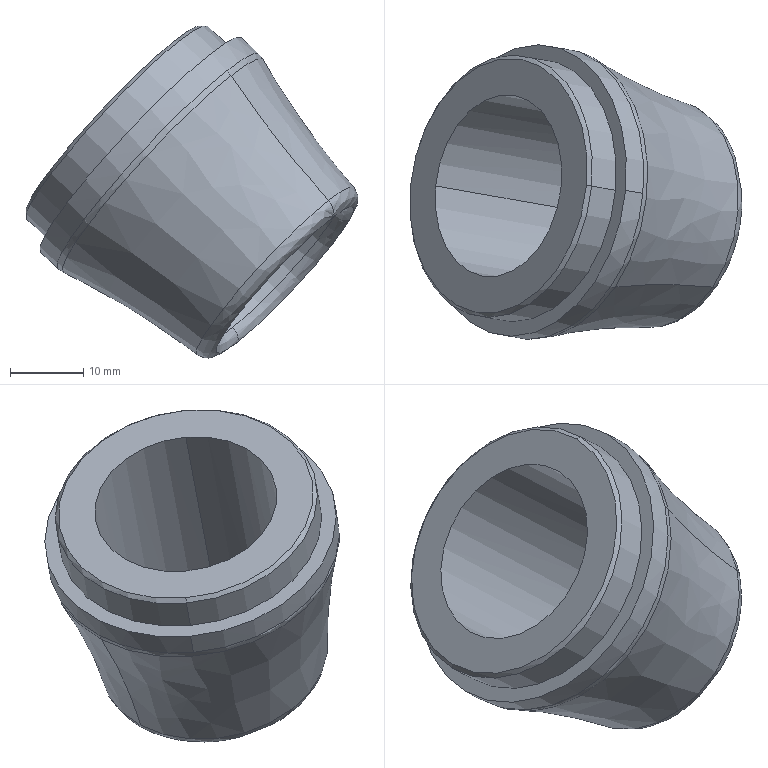Part | SolidWorks | features BaseBody 1 | 1 solid | 18 faces | box 45.219 x 40.115 x 45.273 mm | volume 15947 mm3 | spline 8 | cylinder 4 | cone 4 | plane 2 | commonest cylinder face diameters 25 x2 40 x2
STEP:
#1=CARTESIAN_POINT('',(498.277,-206.019,199.737));
#2=VERTEX_POINT('',#1);
#3=CARTESIAN_POINT('',(485.604,-188.687,182.98));
#4=VERTEX_POINT('',#3);
#5=CARTESIAN_POINT('',(491.94,-197.353,191.359));
#6=DIRECTION('',(0.7235,-0.127,-0.6785));
#7=DIRECTION('',(0.4653,-0.6364,0.6153));
#8=AXIS2_PLACEMENT_3D('',#5,#6,#7);
#9=CIRCLE('',#8,13.618);
#10=EDGE_CURVE('',#2,#4,#9,.T.);
#11=ORIENTED_EDGE('',*,*,#10,.T.);
#12=CARTESIAN_POINT('',(484.825,-189.17,184.886));
#13=VERTEX_POINT('',#12);
#14=CARTESIAN_POINT('',(483.895,-187.898,183.655));
#15=DIRECTION('',(-0.5099,-0.7609,-0.4013));
#16=DIRECTION('',(-0.4653,0.6364,-0.6153));
#17=AXIS2_PLACEMENT_3D('',#14,#15,#16);
#18=CIRCLE('',#17,2.);
#19=EDGE_CURVE('',#4,#13,#18,.T.);
#20=ORIENTED_EDGE('',*,*,#19,.T.);
#21=CARTESIAN_POINT('',(482.091,-197.125,183.459));
#22=VERTEX_POINT('',#21);
#23=CARTESIAN_POINT('',(490.642,-197.125,192.577));
#24=DIRECTION('',(-0.7235,0.127,0.6785));
#25=DIRECTION('',(0.6841,0.,0.7294));
#26=AXIS2_PLACEMENT_3D('',#23,#24,#25);
#27=CIRCLE('',#26,12.5);
#28=EDGE_CURVE('',#13,#22,#27,.T.);
#29=ORIENTED_EDGE('',*,*,#28,.T.);
#30=CARTESIAN_POINT('',(496.458,-205.079,200.267));
#31=VERTEX_POINT('',#30);
#32=CARTESIAN_POINT('',(490.642,-197.125,192.577));
#33=DIRECTION('',(-0.7235,0.127,0.6785));
#34=DIRECTION('',(0.6841,0.,0.7294));
#35=AXIS2_PLACEMENT_3D('',#32,#33,#34);
#36=CIRCLE('',#35,12.5);
#37=EDGE_CURVE('',#22,#31,#36,.T.);
#38=ORIENTED_EDGE('',*,*,#37,.T.);
#39=CARTESIAN_POINT('',(497.389,-206.352,201.498));
#40=DIRECTION('',(0.5099,0.7609,0.4013));
#41=DIRECTION('',(0.4653,-0.6364,0.6153));
#42=AXIS2_PLACEMENT_3D('',#39,#40,#41);
#43=CIRCLE('',#42,2.);
#44=EDGE_CURVE('',#2,#31,#43,.T.);
#45=ORIENTED_EDGE('',*,*,#44,.F.);
#46=EDGE_LOOP('',(#11,#20,#29,#38,#45));
#47=FACE_OUTER_BOUND('',#46,.T.);
#48=CARTESIAN_POINT('',(485.604,-188.687,182.98));
#49=CARTESIAN_POINT('',(471.716,-209.41,172.05));
#50=CARTESIAN_POINT('',(484.389,-226.742,188.807));
#51=CARTESIAN_POINT('',(498.277,-206.019,199.737));
#52=CARTESIAN_POINT('',(485.681,-189.091,183.648));
#53=CARTESIAN_POINT('',(472.511,-208.743,173.282));
#54=CARTESIAN_POINT('',(484.529,-225.179,189.173));
#55=CARTESIAN_POINT('',(497.699,-205.527,199.539));
#56=CARTESIAN_POINT('',(485.392,-189.27,184.354));
#57=CARTESIAN_POINT('',(472.645,-208.292,174.321));
#58=CARTESIAN_POINT('',(484.277,-224.201,189.702));
#59=CARTESIAN_POINT('',(497.025,-205.179,199.735));
#60=CARTESIAN_POINT('',(484.825,-189.17,184.886));
#61=CARTESIAN_POINT('',(472.077,-208.192,174.853));
#62=CARTESIAN_POINT('',(483.71,-224.101,190.234));
#63=CARTESIAN_POINT('',(496.458,-205.079,200.267));
#64=(BOUNDED_SURFACE()B_SPLINE_SURFACE(3,3,((#48,#49,#50,#51),(#52,#53,#54,#55),(#56,#57,#58,#59),(#60,#61,#62,#63)),.UNSPECIFIED.,.F.,.F.,.F.)B_SPLINE_SURFACE_WITH_KNOTS((4,4),(4,4),(0.,1.),(0.,1.),.UNSPECIFIED.)GEOMETRIC_REPRESENTATION_ITEM()RATIONAL_B_SPLINE_SURFACE(((1.,0.3333,0.3333,1.),(0.8992,0.2997,0.2997,0.8992),(0.8992,0.2997,0.2997,0.8992),(1.,0.3333,0.3333,1.)))REPRESENTATION_ITEM('')SURFACE());
#65=ADVANCED_FACE('',(#47),#64,.T.);
#66=CARTESIAN_POINT('',(497.906,-207.057,202.177));
#67=VERTEX_POINT('',#66);
#68=CARTESIAN_POINT('',(483.381,-187.194,182.972));
#69=VERTEX_POINT('',#68);
#70=CARTESIAN_POINT('',(490.644,-197.125,192.575));
#71=DIRECTION('',(0.7235,-0.127,-0.6785));
#72=DIRECTION('',(0.4653,-0.6364,0.6153));
#73=AXIS2_PLACEMENT_3D('',#70,#71,#72);
#74=CIRCLE('',#73,15.607);
#75=EDGE_CURVE('',#67,#69,#74,.T.);
#76=ORIENTED_EDGE('',*,*,#75,.T.);
#77=CARTESIAN_POINT('',(484.157,-188.433,184.337));
#78=DIRECTION('',(-0.5099,-0.7609,-0.4013));
#79=DIRECTION('',(-0.4653,0.6364,-0.6153));
#80=AXIS2_PLACEMENT_3D('',#77,#78,#79);
#81=CIRCLE('',#80,2.);
#82=EDGE_CURVE('',#69,#4,#81,.T.);
#83=ORIENTED_EDGE('',*,*,#82,.T.);
#84=ORIENTED_EDGE('',*,*,#10,.F.);
#85=CARTESIAN_POINT('',(496.83,-205.765,201.094));
#86=DIRECTION('',(0.5099,0.7609,0.4013));
#87=DIRECTION('',(0.4653,-0.6364,0.6153));
#88=AXIS2_PLACEMENT_3D('',#85,#86,#87);
#89=CIRCLE('',#88,2.);
#90=EDGE_CURVE('',#67,#2,#89,.T.);
#91=ORIENTED_EDGE('',*,*,#90,.F.);
#92=EDGE_LOOP('',(#76,#83,#84,#91));
#93=FACE_OUTER_BOUND('',#92,.T.);
#94=CARTESIAN_POINT('',(483.381,-187.194,182.972));
#95=CARTESIAN_POINT('',(467.465,-210.943,170.445));
#96=CARTESIAN_POINT('',(481.989,-230.807,189.65));
#97=CARTESIAN_POINT('',(497.906,-207.057,202.177));
#98=CARTESIAN_POINT('',(484.209,-187.401,182.314));
#99=CARTESIAN_POINT('',(468.406,-210.98,169.877));
#100=CARTESIAN_POINT('',(482.826,-230.702,188.944));
#101=CARTESIAN_POINT('',(498.629,-207.122,201.381));
#102=CARTESIAN_POINT('',(485.103,-188.002,182.317));
#103=CARTESIAN_POINT('',(470.116,-210.363,170.522));
#104=CARTESIAN_POINT('',(483.792,-229.066,188.605));
#105=CARTESIAN_POINT('',(498.778,-206.704,200.4));
#106=CARTESIAN_POINT('',(485.604,-188.687,182.98));
#107=CARTESIAN_POINT('',(471.716,-209.41,172.05));
#108=CARTESIAN_POINT('',(484.389,-226.742,188.807));
#109=CARTESIAN_POINT('',(498.277,-206.019,199.737));
#110=(BOUNDED_SURFACE()B_SPLINE_SURFACE(3,3,((#94,#95,#96,#97),(#98,#99,#100,#101),(#102,#103,#104,#105),(#106,#107,#108,#109)),.UNSPECIFIED.,.F.,.F.,.F.)B_SPLINE_SURFACE_WITH_KNOTS((4,4),(4,4),(0.,1.),(0.,1.),.UNSPECIFIED.)GEOMETRIC_REPRESENTATION_ITEM()RATIONAL_B_SPLINE_SURFACE(((1.,0.3333,0.3333,1.),(0.8286,0.2762,0.2762,0.8286),(0.8286,0.2762,0.2762,0.8286),(1.,0.3333,0.3333,1.)))REPRESENTATION_ITEM('')SURFACE());
#111=ADVANCED_FACE('',(#93),#110,.T.);
#112=CARTESIAN_POINT('',(490.644,-197.125,192.575));
#113=DIRECTION('',(0.7235,-0.127,-0.6785));
#114=DIRECTION('',(0.4653,-0.6364,0.6153));
#115=AXIS2_PLACEMENT_3D('',#112,#113,#114);
#116=CIRCLE('',#115,15.607);
#117=EDGE_CURVE('',#69,#67,#116,.T.);
#118=ORIENTED_EDGE('',*,*,#117,.F.);
#119=CARTESIAN_POINT('',(466.115,-181.798,194.681));
#120=VERTEX_POINT('',#119);
#121=CARTESIAN_POINT('',(439.429,-116.93,105.607));
#122=DIRECTION('',(-0.5099,-0.7609,-0.4013));
#123=DIRECTION('',(-0.4653,0.6364,-0.6153));
#124=AXIS2_PLACEMENT_3D('',#121,#122,#123);
#125=CIRCLE('',#124,113.377);
#126=EDGE_CURVE('',#69,#120,#125,.T.);
#127=ORIENTED_EDGE('',*,*,#126,.T.);
#128=CARTESIAN_POINT('',(484.608,-207.088,219.132));
#129=VERTEX_POINT('',#128);
#130=CARTESIAN_POINT('',(475.361,-194.443,206.907));
#131=DIRECTION('',(-0.7235,0.127,0.6785));
#132=DIRECTION('',(0.4653,-0.6364,0.6153));
#133=AXIS2_PLACEMENT_3D('',#130,#131,#132);
#134=CIRCLE('',#133,19.871);
#135=EDGE_CURVE('',#129,#120,#134,.T.);
#136=ORIENTED_EDGE('',*,*,#135,.F.);
#137=CARTESIAN_POINT('',(558.893,-280.31,263.568));
#138=DIRECTION('',(0.5099,0.7609,0.4013));
#139=DIRECTION('',(0.4653,-0.6364,0.6153));
#140=AXIS2_PLACEMENT_3D('',#137,#138,#139);
#141=CIRCLE('',#140,113.377);
#142=EDGE_CURVE('',#67,#129,#141,.T.);
#143=ORIENTED_EDGE('',*,*,#142,.F.);
#144=EDGE_LOOP('',(#118,#127,#136,#143));
#145=FACE_OUTER_BOUND('',#144,.T.);
#146=CARTESIAN_POINT('',(497.906,-207.057,202.177));
#147=CARTESIAN_POINT('',(513.822,-183.307,214.704));
#148=CARTESIAN_POINT('',(499.298,-163.444,195.5));
#149=CARTESIAN_POINT('',(483.381,-187.194,182.972));
#150=CARTESIAN_POINT('',(493.069,-206.623,207.499));
#151=CARTESIAN_POINT('',(509.749,-181.735,220.627));
#152=CARTESIAN_POINT('',(494.529,-160.919,200.502));
#153=CARTESIAN_POINT('',(477.849,-185.808,187.374));
#154=CARTESIAN_POINT('',(488.623,-206.634,213.168));
#155=CARTESIAN_POINT('',(506.757,-179.576,227.44));
#156=CARTESIAN_POINT('',(490.21,-156.946,205.561));
#157=CARTESIAN_POINT('',(472.076,-184.004,191.289));
#158=CARTESIAN_POINT('',(484.608,-207.088,219.132));
#159=CARTESIAN_POINT('',(504.873,-176.85,235.082));
#160=CARTESIAN_POINT('',(486.38,-151.56,210.631));
#161=CARTESIAN_POINT('',(466.115,-181.798,194.681));
#162=(BOUNDED_SURFACE()B_SPLINE_SURFACE(3,3,((#146,#147,#148,#149),(#150,#151,#152,#153),(#154,#155,#156,#157),(#158,#159,#160,#161)),.UNSPECIFIED.,.F.,.F.,.F.)B_SPLINE_SURFACE_WITH_KNOTS((4,4),(4,4),(0.,1.),(0.,1.),.UNSPECIFIED.)GEOMETRIC_REPRESENTATION_ITEM()RATIONAL_B_SPLINE_SURFACE(((1.,0.3333,0.3333,1.),(0.997,0.3323,0.3323,0.997),(0.997,0.3323,0.3323,0.997),(1.,0.3333,0.3333,1.)))REPRESENTATION_ITEM('')SURFACE());
#163=ADVANCED_FACE('',(#145),#162,.F.);
#164=CARTESIAN_POINT('',(461.05,-194.333,192.909));
#165=VERTEX_POINT('',#164);
#166=CARTESIAN_POINT('',(465.425,-181.605,195.192));
#167=VERTEX_POINT('',#166);
#168=CARTESIAN_POINT('',(474.732,-194.333,207.497));
#169=DIRECTION('',(0.7235,-0.127,-0.6785));
#170=DIRECTION('',(0.4653,-0.6364,0.6153));
#171=AXIS2_PLACEMENT_3D('',#168,#169,#170);
#172=CIRCLE('',#171,20.);
#173=EDGE_CURVE('',#165,#167,#172,.T.);
#174=ORIENTED_EDGE('',*,*,#173,.T.);
#175=CARTESIAN_POINT('',(466.821,-183.514,197.038));
#176=DIRECTION('',(-0.5099,-0.7609,-0.4013));
#177=DIRECTION('',(-0.4653,0.6364,-0.6153));
#178=AXIS2_PLACEMENT_3D('',#175,#176,#177);
#179=CIRCLE('',#178,3.);
#180=EDGE_CURVE('',#167,#120,#179,.T.);
#181=ORIENTED_EDGE('',*,*,#180,.T.);
#182=CARTESIAN_POINT('',(475.361,-194.443,206.907));
#183=DIRECTION('',(-0.7235,0.127,0.6785));
#184=DIRECTION('',(0.4653,-0.6364,0.6153));
#185=AXIS2_PLACEMENT_3D('',#182,#183,#184);
#186=CIRCLE('',#185,19.871);
#187=EDGE_CURVE('',#120,#129,#186,.T.);
#188=ORIENTED_EDGE('',*,*,#187,.T.);
#189=CARTESIAN_POINT('',(484.038,-207.06,219.802));
#190=VERTEX_POINT('',#189);
#191=CARTESIAN_POINT('',(482.642,-205.151,217.957));
#192=DIRECTION('',(0.5099,0.7609,0.4013));
#193=DIRECTION('',(0.4653,-0.6364,0.6153));
#194=AXIS2_PLACEMENT_3D('',#191,#192,#193);
#195=CIRCLE('',#194,3.);
#196=EDGE_CURVE('',#190,#129,#195,.T.);
#197=ORIENTED_EDGE('',*,*,#196,.F.);
#198=CARTESIAN_POINT('',(474.732,-194.333,207.497));
#199=DIRECTION('',(0.7235,-0.127,-0.6785));
#200=DIRECTION('',(0.4653,-0.6364,0.6153));
#201=AXIS2_PLACEMENT_3D('',#198,#199,#200);
#202=CIRCLE('',#201,20.);
#203=EDGE_CURVE('',#190,#165,#202,.T.);
#204=ORIENTED_EDGE('',*,*,#203,.T.);
#205=EDGE_LOOP('',(#174,#181,#188,#197,#204));
#206=FACE_OUTER_BOUND('',#205,.T.);
#207=CARTESIAN_POINT('',(465.425,-181.605,195.192));
#208=CARTESIAN_POINT('',(445.029,-212.04,179.139));
#209=CARTESIAN_POINT('',(463.641,-237.494,203.749));
#210=CARTESIAN_POINT('',(484.038,-207.06,219.802));
#211=CARTESIAN_POINT('',(465.639,-181.643,194.992));
#212=CARTESIAN_POINT('',(445.243,-212.078,178.939));
#213=CARTESIAN_POINT('',(463.855,-237.532,203.549));
#214=CARTESIAN_POINT('',(484.252,-207.097,219.602));
#215=CARTESIAN_POINT('',(465.871,-181.708,194.82));
#216=CARTESIAN_POINT('',(445.518,-212.076,178.802));
#217=CARTESIAN_POINT('',(464.09,-237.476,203.359));
#218=CARTESIAN_POINT('',(484.443,-207.107,219.377));
#219=CARTESIAN_POINT('',(466.115,-181.798,194.681));
#220=CARTESIAN_POINT('',(445.85,-212.036,178.732));
#221=CARTESIAN_POINT('',(464.342,-237.327,203.183));
#222=CARTESIAN_POINT('',(484.608,-207.088,219.132));
#223=(BOUNDED_SURFACE()B_SPLINE_SURFACE(3,3,((#207,#208,#209,#210),(#211,#212,#213,#214),(#215,#216,#217,#218),(#219,#220,#221,#222)),.UNSPECIFIED.,.F.,.F.,.T.)B_SPLINE_SURFACE_WITH_KNOTS((4,4),(4,4),(0.,1.),(0.,1.),.UNSPECIFIED.)GEOMETRIC_REPRESENTATION_ITEM()RATIONAL_B_SPLINE_SURFACE(((1.,0.3333,0.3333,1.),(0.9928,0.3309,0.3309,0.9928),(0.9928,0.3309,0.3309,0.9928),(1.,0.3333,0.3333,1.)))REPRESENTATION_ITEM('')SURFACE());
#224=ADVANCED_FACE('',(#206),#223,.T.);
#225=ORIENTED_EDGE('',*,*,#37,.F.);
#226=CARTESIAN_POINT('',(460.203,-193.283,203.985));
#227=VERTEX_POINT('',#226);
#228=CARTESIAN_POINT('',(483.39,-197.353,182.241));
#229=DIRECTION('',(-0.7235,0.127,0.6785));
#230=VECTOR('',#229,1000.);
#231=LINE('',#228,#230);
#232=EDGE_CURVE('',#22,#227,#231,.T.);
#233=ORIENTED_EDGE('',*,*,#232,.T.);
#234=CARTESIAN_POINT('',(477.305,-193.283,222.221));
#235=VERTEX_POINT('',#234);
#236=CARTESIAN_POINT('',(468.754,-193.283,213.103));
#237=DIRECTION('',(0.7235,-0.127,-0.6785));
#238=DIRECTION('',(0.6841,0.,0.7294));
#239=AXIS2_PLACEMENT_3D('',#236,#237,#238);
#240=CIRCLE('',#239,12.5);
#241=EDGE_CURVE('',#235,#227,#240,.T.);
#242=ORIENTED_EDGE('',*,*,#241,.F.);
#243=CARTESIAN_POINT('',(499.193,-197.125,201.694));
#244=VERTEX_POINT('',#243);
#245=CARTESIAN_POINT('',(500.491,-197.353,200.476));
#246=DIRECTION('',(-0.7235,0.127,0.6785));
#247=VECTOR('',#246,1000.);
#248=LINE('',#245,#247);
#249=EDGE_CURVE('',#244,#235,#248,.T.);
#250=ORIENTED_EDGE('',*,*,#249,.F.);
#251=CARTESIAN_POINT('',(490.642,-197.125,192.577));
#252=DIRECTION('',(-0.7235,0.127,0.6785));
#253=DIRECTION('',(0.6841,0.,0.7294));
#254=AXIS2_PLACEMENT_3D('',#251,#252,#253);
#255=CIRCLE('',#254,12.5);
#256=EDGE_CURVE('',#31,#244,#255,.T.);
#257=ORIENTED_EDGE('',*,*,#256,.F.);
#258=EDGE_LOOP('',(#225,#233,#242,#250,#257));
#259=FACE_OUTER_BOUND('',#258,.T.);
#260=CARTESIAN_POINT('',(491.94,-197.353,191.359));
#261=DIRECTION('',(-0.7235,0.127,0.6785));
#262=DIRECTION('',(0.6841,0.,0.7294));
#263=AXIS2_PLACEMENT_3D('',#260,#261,#262);
#264=CYLINDRICAL_SURFACE('',#263,12.5);
#265=ADVANCED_FACE('',(#259),#264,.F.);
#266=CARTESIAN_POINT('',(456.784,-193.283,200.339));
#267=VERTEX_POINT('',#266);
#268=CARTESIAN_POINT('',(480.725,-193.283,225.867));
#269=VERTEX_POINT('',#268);
#270=CARTESIAN_POINT('',(468.754,-193.283,213.103));
#271=DIRECTION('',(0.7235,-0.127,-0.6785));
#272=DIRECTION('',(-0.6841,0.,-0.7294));
#273=AXIS2_PLACEMENT_3D('',#270,#271,#272);
#274=CIRCLE('',#273,17.499);
#275=EDGE_CURVE('',#267,#269,#274,.T.);
#276=ORIENTED_EDGE('',*,*,#275,.T.);
#277=CARTESIAN_POINT('',(481.429,-193.347,225.893));
#278=VERTEX_POINT('',#277);
#279=CARTESIAN_POINT('',(481.429,-193.347,225.893));
#280=DIRECTION('',(0.9953,-0.08978,0.03607));
#281=VECTOR('',#280,1000.);
#282=LINE('',#279,#281);
#283=EDGE_CURVE('',#269,#278,#282,.T.);
#284=ORIENTED_EDGE('',*,*,#283,.T.);
#285=CARTESIAN_POINT('',(456.803,-193.347,199.635));
#286=VERTEX_POINT('',#285);
#287=CARTESIAN_POINT('',(469.116,-193.347,212.764));
#288=DIRECTION('',(-0.7235,0.127,0.6785));
#289=DIRECTION('',(-0.4653,0.6364,-0.6153));
#290=AXIS2_PLACEMENT_3D('',#287,#288,#289);
#291=CIRCLE('',#290,17.999);
#292=EDGE_CURVE('',#278,#286,#291,.T.);
#293=ORIENTED_EDGE('',*,*,#292,.T.);
#294=CARTESIAN_POINT('',(456.803,-193.347,199.635));
#295=DIRECTION('',(0.02781,-0.08978,-0.9956));
#296=VECTOR('',#295,1000.);
#297=LINE('',#294,#296);
#298=EDGE_CURVE('',#267,#286,#297,.T.);
#299=ORIENTED_EDGE('',*,*,#298,.F.);
#300=EDGE_LOOP('',(#276,#284,#293,#299));
#301=FACE_OUTER_BOUND('',#300,.T.);
#302=CARTESIAN_POINT('',(469.116,-193.347,212.764));
#303=DIRECTION('',(0.7235,-0.127,-0.6785));
#304=DIRECTION('',(-0.6841,0.,-0.7294));
#305=AXIS2_PLACEMENT_3D('',#302,#303,#304);
#306=CONICAL_SURFACE('',#305,17.999,0.7855);
#307=ADVANCED_FACE('',(#301),#306,.T.);
#308=ORIENTED_EDGE('',*,*,#292,.F.);
#309=CARTESIAN_POINT('',(484.685,-193.918,222.84));
#310=VERTEX_POINT('',#309);
#311=CARTESIAN_POINT('',(484.685,-193.918,222.84));
#312=DIRECTION('',(0.7236,-0.127,-0.6784));
#313=VECTOR('',#312,1000.);
#314=LINE('',#311,#313);
#315=EDGE_CURVE('',#278,#310,#314,.T.);
#316=ORIENTED_EDGE('',*,*,#315,.T.);
#317=CARTESIAN_POINT('',(460.059,-193.918,196.581));
#318=VERTEX_POINT('',#317);
#319=CARTESIAN_POINT('',(472.372,-193.918,209.71));
#320=DIRECTION('',(-0.7235,0.127,0.6785));
#321=DIRECTION('',(-0.6841,0.,-0.7294));
#322=AXIS2_PLACEMENT_3D('',#319,#320,#321);
#323=CIRCLE('',#322,18.);
#324=EDGE_CURVE('',#310,#318,#323,.T.);
#325=ORIENTED_EDGE('',*,*,#324,.T.);
#326=CARTESIAN_POINT('',(460.059,-193.918,196.581));
#327=DIRECTION('',(0.7234,-0.127,-0.6787));
#328=VECTOR('',#327,1000.);
#329=LINE('',#326,#328);
#330=EDGE_CURVE('',#286,#318,#329,.T.);
#331=ORIENTED_EDGE('',*,*,#330,.F.);
#332=EDGE_LOOP('',(#308,#316,#325,#331));
#333=FACE_OUTER_BOUND('',#332,.T.);
#334=CARTESIAN_POINT('',(472.372,-193.918,209.71));
#335=DIRECTION('',(0.7235,-0.127,-0.6785));
#336=DIRECTION('',(-0.6841,0.,-0.7294));
#337=AXIS2_PLACEMENT_3D('',#334,#335,#336);
#338=CONICAL_SURFACE('',#337,18.,0.0001745);
#339=ADVANCED_FACE('',(#333),#338,.T.);
#340=CARTESIAN_POINT('',(458.691,-193.918,195.122));
#341=VERTEX_POINT('',#340);
#342=CARTESIAN_POINT('',(486.053,-193.918,224.299));
#343=VERTEX_POINT('',#342);
#344=CARTESIAN_POINT('',(472.372,-193.918,209.71));
#345=DIRECTION('',(0.7235,-0.127,-0.6785));
#346=DIRECTION('',(-0.6841,0.,-0.7294));
#347=AXIS2_PLACEMENT_3D('',#344,#345,#346);
#348=CIRCLE('',#347,20.);
#349=EDGE_CURVE('',#341,#343,#348,.T.);
#350=ORIENTED_EDGE('',*,*,#349,.T.);
#351=CARTESIAN_POINT('',(488.413,-194.333,222.086));
#352=VERTEX_POINT('',#351);
#353=CARTESIAN_POINT('',(487.395,-194.154,223.04));
#354=DIRECTION('',(0.7235,-0.127,-0.6785));
#355=VECTOR('',#354,1000.);
#356=LINE('',#353,#355);
#357=EDGE_CURVE('',#343,#352,#356,.T.);
#358=ORIENTED_EDGE('',*,*,#357,.T.);
#359=CARTESIAN_POINT('',(474.732,-194.333,207.497));
#360=DIRECTION('',(0.7235,-0.127,-0.6785));
#361=DIRECTION('',(0.4653,-0.6364,0.6153));
#362=AXIS2_PLACEMENT_3D('',#359,#360,#361);
#363=CIRCLE('',#362,20.);
#364=EDGE_CURVE('',#167,#352,#363,.T.);
#365=ORIENTED_EDGE('',*,*,#364,.F.);
#366=ORIENTED_EDGE('',*,*,#173,.F.);
#367=CARTESIAN_POINT('',(460.032,-194.154,193.864));
#368=DIRECTION('',(0.7235,-0.127,-0.6785));
#369=VECTOR('',#368,1000.);
#370=LINE('',#367,#369);
#371=EDGE_CURVE('',#341,#165,#370,.T.);
#372=ORIENTED_EDGE('',*,*,#371,.F.);
#373=EDGE_LOOP('',(#350,#358,#365,#366,#372));
#374=FACE_OUTER_BOUND('',#373,.T.);
#375=CARTESIAN_POINT('',(473.714,-194.154,208.452));
#376=DIRECTION('',(0.7235,-0.127,-0.6785));
#377=DIRECTION('',(-0.6841,0.,-0.7294));
#378=AXIS2_PLACEMENT_3D('',#375,#376,#377);
#379=CYLINDRICAL_SURFACE('',#378,20.);
#380=ADVANCED_FACE('',(#374),#379,.T.);
#381=ORIENTED_EDGE('',*,*,#232,.F.);
#382=ORIENTED_EDGE('',*,*,#28,.F.);
#383=CARTESIAN_POINT('',(490.642,-197.125,192.577));
#384=DIRECTION('',(-0.7235,0.127,0.6785));
#385=DIRECTION('',(0.6841,0.,0.7294));
#386=AXIS2_PLACEMENT_3D('',#383,#384,#385);
#387=CIRCLE('',#386,12.5);
#388=EDGE_CURVE('',#244,#13,#387,.T.);
#389=ORIENTED_EDGE('',*,*,#388,.F.);
#390=ORIENTED_EDGE('',*,*,#249,.T.);
#391=CARTESIAN_POINT('',(468.754,-193.283,213.103));
#392=DIRECTION('',(0.7235,-0.127,-0.6785));
#393=DIRECTION('',(0.6841,0.,0.7294));
#394=AXIS2_PLACEMENT_3D('',#391,#392,#393);
#395=CIRCLE('',#394,12.5);
#396=EDGE_CURVE('',#227,#235,#395,.T.);
#397=ORIENTED_EDGE('',*,*,#396,.F.);
#398=EDGE_LOOP('',(#381,#382,#389,#390,#397));
#399=FACE_OUTER_BOUND('',#398,.T.);
#400=CARTESIAN_POINT('',(491.94,-197.353,191.359));
#401=DIRECTION('',(-0.7235,0.127,0.6785));
#402=DIRECTION('',(0.6841,0.,0.7294));
#403=AXIS2_PLACEMENT_3D('',#400,#401,#402);
#404=CYLINDRICAL_SURFACE('',#403,12.5);
#405=ADVANCED_FACE('',(#399),#404,.F.);
#406=ORIENTED_EDGE('',*,*,#19,.F.);
#407=CARTESIAN_POINT('',(491.94,-197.353,191.359));
#408=DIRECTION('',(0.7235,-0.127,-0.6785));
#409=DIRECTION('',(0.4653,-0.6364,0.6153));
#410=AXIS2_PLACEMENT_3D('',#407,#408,#409);
#411=CIRCLE('',#410,13.618);
#412=EDGE_CURVE('',#4,#2,#411,.T.);
#413=ORIENTED_EDGE('',*,*,#412,.T.);
#414=ORIENTED_EDGE('',*,*,#44,.T.);
#415=ORIENTED_EDGE('',*,*,#256,.T.);
#416=ORIENTED_EDGE('',*,*,#388,.T.);
#417=EDGE_LOOP('',(#406,#413,#414,#415,#416));
#418=FACE_OUTER_BOUND('',#417,.T.);
#419=CARTESIAN_POINT('',(498.277,-206.019,199.737));
#420=CARTESIAN_POINT('',(512.165,-185.296,210.668));
#421=CARTESIAN_POINT('',(499.492,-167.964,193.911));
#422=CARTESIAN_POINT('',(485.604,-188.687,182.98));
#423=CARTESIAN_POINT('',(497.699,-205.527,199.539));
#424=CARTESIAN_POINT('',(510.87,-185.875,209.905));
#425=CARTESIAN_POINT('',(498.852,-169.438,194.013));
#426=CARTESIAN_POINT('',(485.681,-189.091,183.648));
#427=CARTESIAN_POINT('',(497.025,-205.179,199.735));
#428=CARTESIAN_POINT('',(509.773,-186.157,209.769));
#429=CARTESIAN_POINT('',(498.14,-170.248,194.387));
#430=CARTESIAN_POINT('',(485.392,-189.27,184.354));
#431=CARTESIAN_POINT('',(496.458,-205.079,200.267));
#432=CARTESIAN_POINT('',(509.206,-186.058,210.3));
#433=CARTESIAN_POINT('',(497.573,-170.149,194.919));
#434=CARTESIAN_POINT('',(484.825,-189.17,184.886));
#435=(BOUNDED_SURFACE()B_SPLINE_SURFACE(3,3,((#419,#420,#421,#422),(#423,#424,#425,#426),(#427,#428,#429,#430),(#431,#432,#433,#434)),.UNSPECIFIED.,.F.,.F.,.T.)B_SPLINE_SURFACE_WITH_KNOTS((4,4),(4,4),(0.,1.),(0.,1.),.UNSPECIFIED.)GEOMETRIC_REPRESENTATION_ITEM()RATIONAL_B_SPLINE_SURFACE(((1.,0.3333,0.3333,1.),(0.8992,0.2997,0.2997,0.8992),(0.8992,0.2997,0.2997,0.8992),(1.,0.3333,0.3333,1.)))REPRESENTATION_ITEM('')SURFACE());
#436=ADVANCED_FACE('',(#418),#435,.T.);
#437=ORIENTED_EDGE('',*,*,#275,.F.);
#438=CARTESIAN_POINT('',(468.754,-193.283,213.103));
#439=DIRECTION('',(0.7235,-0.127,-0.6785));
#440=DIRECTION('',(-0.6841,0.,-0.7294));
#441=AXIS2_PLACEMENT_3D('',#438,#439,#440);
#442=CIRCLE('',#441,17.499);
#443=EDGE_CURVE('',#269,#267,#442,.T.);
#444=ORIENTED_EDGE('',*,*,#443,.F.);
#445=EDGE_LOOP('',(#437,#444));
#446=FACE_OUTER_BOUND('',#445,.T.);
#447=ORIENTED_EDGE('',*,*,#241,.T.);
#448=ORIENTED_EDGE('',*,*,#396,.T.);
#449=EDGE_LOOP('',(#447,#448));
#450=FACE_BOUND('',#449,.T.);
#451=CARTESIAN_POINT('',(468.754,-193.283,213.103));
#452=DIRECTION('',(0.7235,-0.127,-0.6785));
#453=DIRECTION('',(-0.6841,0.,-0.7294));
#454=AXIS2_PLACEMENT_3D('',#451,#452,#453);
#455=PLANE('',#454);
#456=ADVANCED_FACE('',(#446,#450),#455,.F.);
#457=ORIENTED_EDGE('',*,*,#82,.F.);
#458=ORIENTED_EDGE('',*,*,#117,.T.);
#459=ORIENTED_EDGE('',*,*,#90,.T.);
#460=ORIENTED_EDGE('',*,*,#412,.F.);
#461=EDGE_LOOP('',(#457,#458,#459,#460));
#462=FACE_OUTER_BOUND('',#461,.T.);
#463=CARTESIAN_POINT('',(497.906,-207.057,202.177));
#464=CARTESIAN_POINT('',(513.822,-183.307,214.704));
#465=CARTESIAN_POINT('',(499.298,-163.444,195.5));
#466=CARTESIAN_POINT('',(483.381,-187.194,182.972));
#467=CARTESIAN_POINT('',(498.629,-207.122,201.381));
#468=CARTESIAN_POINT('',(514.431,-183.542,213.819));
#469=CARTESIAN_POINT('',(500.011,-163.821,194.752));
#470=CARTESIAN_POINT('',(484.209,-187.401,182.314));
#471=CARTESIAN_POINT('',(498.778,-206.704,200.4));
#472=CARTESIAN_POINT('',(513.765,-184.342,212.195));
#473=CARTESIAN_POINT('',(500.089,-165.64,194.113));
#474=CARTESIAN_POINT('',(485.103,-188.002,182.317));
#475=CARTESIAN_POINT('',(498.277,-206.019,199.737));
#476=CARTESIAN_POINT('',(512.165,-185.296,210.668));
#477=CARTESIAN_POINT('',(499.492,-167.964,193.911));
#478=CARTESIAN_POINT('',(485.604,-188.687,182.98));
#479=(BOUNDED_SURFACE()B_SPLINE_SURFACE(3,3,((#463,#464,#465,#466),(#467,#468,#469,#470),(#471,#472,#473,#474),(#475,#476,#477,#478)),.UNSPECIFIED.,.F.,.F.,.T.)B_SPLINE_SURFACE_WITH_KNOTS((4,4),(4,4),(0.,1.),(0.,1.),.UNSPECIFIED.)GEOMETRIC_REPRESENTATION_ITEM()RATIONAL_B_SPLINE_SURFACE(((1.,0.3333,0.3333,1.),(0.8286,0.2762,0.2762,0.8286),(0.8286,0.2762,0.2762,0.8286),(1.,0.3333,0.3333,1.)))REPRESENTATION_ITEM('')SURFACE());
#480=ADVANCED_FACE('',(#462),#479,.T.);
#481=ORIENTED_EDGE('',*,*,#283,.F.);
#482=ORIENTED_EDGE('',*,*,#443,.T.);
#483=ORIENTED_EDGE('',*,*,#298,.T.);
#484=CARTESIAN_POINT('',(469.116,-193.347,212.764));
#485=DIRECTION('',(-0.7235,0.127,0.6785));
#486=DIRECTION('',(-0.4653,0.6364,-0.6153));
#487=AXIS2_PLACEMENT_3D('',#484,#485,#486);
#488=CIRCLE('',#487,17.999);
#489=EDGE_CURVE('',#286,#278,#488,.T.);
#490=ORIENTED_EDGE('',*,*,#489,.T.);
#491=EDGE_LOOP('',(#481,#482,#483,#490));
#492=FACE_OUTER_BOUND('',#491,.T.);
#493=CARTESIAN_POINT('',(469.116,-193.347,212.764));
#494=DIRECTION('',(0.7235,-0.127,-0.6785));
#495=DIRECTION('',(-0.6841,0.,-0.7294));
#496=AXIS2_PLACEMENT_3D('',#493,#494,#495);
#497=CONICAL_SURFACE('',#496,17.999,0.7855);
#498=ADVANCED_FACE('',(#492),#497,.T.);
#499=ORIENTED_EDGE('',*,*,#126,.F.);
#500=ORIENTED_EDGE('',*,*,#75,.F.);
#501=ORIENTED_EDGE('',*,*,#142,.T.);
#502=ORIENTED_EDGE('',*,*,#187,.F.);
#503=EDGE_LOOP('',(#499,#500,#501,#502));
#504=FACE_OUTER_BOUND('',#503,.T.);
#505=CARTESIAN_POINT('',(483.381,-187.194,182.972));
#506=CARTESIAN_POINT('',(467.465,-210.943,170.445));
#507=CARTESIAN_POINT('',(481.989,-230.807,189.65));
#508=CARTESIAN_POINT('',(497.906,-207.057,202.177));
#509=CARTESIAN_POINT('',(477.849,-185.808,187.374));
#510=CARTESIAN_POINT('',(461.17,-210.696,174.247));
#511=CARTESIAN_POINT('',(476.39,-231.511,194.372));
#512=CARTESIAN_POINT('',(493.069,-206.623,207.499));
#513=CARTESIAN_POINT('',(472.076,-184.004,191.289));
#514=CARTESIAN_POINT('',(453.943,-211.061,177.017));
#515=CARTESIAN_POINT('',(470.49,-233.691,198.896));
#516=CARTESIAN_POINT('',(488.623,-206.634,213.168));
#517=CARTESIAN_POINT('',(466.115,-181.798,194.681));
#518=CARTESIAN_POINT('',(445.85,-212.036,178.732));
#519=CARTESIAN_POINT('',(464.342,-237.327,203.183));
#520=CARTESIAN_POINT('',(484.608,-207.088,219.132));
#521=(BOUNDED_SURFACE()B_SPLINE_SURFACE(3,3,((#505,#506,#507,#508),(#509,#510,#511,#512),(#513,#514,#515,#516),(#517,#518,#519,#520)),.UNSPECIFIED.,.F.,.F.,.F.)B_SPLINE_SURFACE_WITH_KNOTS((4,4),(4,4),(0.,1.),(0.,1.),.UNSPECIFIED.)GEOMETRIC_REPRESENTATION_ITEM()RATIONAL_B_SPLINE_SURFACE(((1.,0.3333,0.3333,1.),(0.997,0.3323,0.3323,0.997),(0.997,0.3323,0.3323,0.997),(1.,0.3333,0.3333,1.)))REPRESENTATION_ITEM('')SURFACE());
#522=ADVANCED_FACE('',(#504),#521,.F.);
#523=ORIENTED_EDGE('',*,*,#315,.F.);
#524=ORIENTED_EDGE('',*,*,#489,.F.);
#525=ORIENTED_EDGE('',*,*,#330,.T.);
#526=CARTESIAN_POINT('',(472.372,-193.918,209.71));
#527=DIRECTION('',(-0.7235,0.127,0.6785));
#528=DIRECTION('',(-0.6841,0.,-0.7294));
#529=AXIS2_PLACEMENT_3D('',#526,#527,#528);
#530=CIRCLE('',#529,18.);
#531=EDGE_CURVE('',#318,#310,#530,.T.);
#532=ORIENTED_EDGE('',*,*,#531,.T.);
#533=EDGE_LOOP('',(#523,#524,#525,#532));
#534=FACE_OUTER_BOUND('',#533,.T.);
#535=CARTESIAN_POINT('',(472.372,-193.918,209.71));
#536=DIRECTION('',(0.7235,-0.127,-0.6785));
#537=DIRECTION('',(-0.6841,0.,-0.7294));
#538=AXIS2_PLACEMENT_3D('',#535,#536,#537);
#539=CONICAL_SURFACE('',#538,18.,0.0001745);
#540=ADVANCED_FACE('',(#534),#539,.T.);
#541=ORIENTED_EDGE('',*,*,#180,.F.);
#542=ORIENTED_EDGE('',*,*,#364,.T.);
#543=CARTESIAN_POINT('',(474.732,-194.333,207.497));
#544=DIRECTION('',(0.7235,-0.127,-0.6785));
#545=DIRECTION('',(0.4653,-0.6364,0.6153));
#546=AXIS2_PLACEMENT_3D('',#543,#544,#545);
#547=CIRCLE('',#546,20.);
#548=EDGE_CURVE('',#352,#190,#547,.T.);
#549=ORIENTED_EDGE('',*,*,#548,.T.);
#550=ORIENTED_EDGE('',*,*,#196,.T.);
#551=ORIENTED_EDGE('',*,*,#135,.T.);
#552=EDGE_LOOP('',(#541,#542,#549,#550,#551));
#553=FACE_OUTER_BOUND('',#552,.T.);
#554=CARTESIAN_POINT('',(484.038,-207.06,219.802));
#555=CARTESIAN_POINT('',(504.434,-176.625,235.856));
#556=CARTESIAN_POINT('',(485.822,-151.171,211.245));
#557=CARTESIAN_POINT('',(465.425,-181.605,195.192));
#558=CARTESIAN_POINT('',(484.252,-207.097,219.602));
#559=CARTESIAN_POINT('',(504.648,-176.663,235.655));
#560=CARTESIAN_POINT('',(486.036,-151.208,211.045));
#561=CARTESIAN_POINT('',(465.639,-181.643,194.992));
#562=CARTESIAN_POINT('',(484.443,-207.107,219.377));
#563=CARTESIAN_POINT('',(504.795,-176.738,235.395));
#564=CARTESIAN_POINT('',(486.223,-151.339,210.839));
#565=CARTESIAN_POINT('',(465.871,-181.708,194.82));
#566=CARTESIAN_POINT('',(484.608,-207.088,219.132));
#567=CARTESIAN_POINT('',(504.873,-176.85,235.082));
#568=CARTESIAN_POINT('',(486.38,-151.56,210.631));
#569=CARTESIAN_POINT('',(466.115,-181.798,194.681));
#570=(BOUNDED_SURFACE()B_SPLINE_SURFACE(3,3,((#554,#555,#556,#557),(#558,#559,#560,#561),(#562,#563,#564,#565),(#566,#567,#568,#569)),.UNSPECIFIED.,.F.,.F.,.F.)B_SPLINE_SURFACE_WITH_KNOTS((4,4),(4,4),(0.,1.),(0.,1.),.UNSPECIFIED.)GEOMETRIC_REPRESENTATION_ITEM()RATIONAL_B_SPLINE_SURFACE(((1.,0.3333,0.3333,1.),(0.9928,0.3309,0.3309,0.9928),(0.9928,0.3309,0.3309,0.9928),(1.,0.3333,0.3333,1.)))REPRESENTATION_ITEM('')SURFACE());
#571=ADVANCED_FACE('',(#553),#570,.T.);
#572=ORIENTED_EDGE('',*,*,#531,.F.);
#573=ORIENTED_EDGE('',*,*,#324,.F.);
#574=EDGE_LOOP('',(#572,#573));
#575=FACE_BOUND('',#574,.T.);
#576=ORIENTED_EDGE('',*,*,#349,.F.);
#577=CARTESIAN_POINT('',(472.372,-193.918,209.71));
#578=DIRECTION('',(0.7235,-0.127,-0.6785));
#579=DIRECTION('',(-0.6841,0.,-0.7294));
#580=AXIS2_PLACEMENT_3D('',#577,#578,#579);
#581=CIRCLE('',#580,20.);
#582=EDGE_CURVE('',#343,#341,#581,.T.);
#583=ORIENTED_EDGE('',*,*,#582,.F.);
#584=EDGE_LOOP('',(#576,#583));
#585=FACE_OUTER_BOUND('',#584,.T.);
#586=CARTESIAN_POINT('',(477.025,-200.282,215.863));
#587=DIRECTION('',(0.7235,-0.127,-0.6785));
#588=DIRECTION('',(-0.6841,0.,-0.7294));
#589=AXIS2_PLACEMENT_3D('',#586,#587,#588);
#590=PLANE('',#589);
#591=ADVANCED_FACE('',(#575,#585),#590,.F.);
#592=ORIENTED_EDGE('',*,*,#357,.F.);
#593=ORIENTED_EDGE('',*,*,#582,.T.);
#594=ORIENTED_EDGE('',*,*,#371,.T.);
#595=ORIENTED_EDGE('',*,*,#203,.F.);
#596=ORIENTED_EDGE('',*,*,#548,.F.);
#597=EDGE_LOOP('',(#592,#593,#594,#595,#596));
#598=FACE_OUTER_BOUND('',#597,.T.);
#599=CARTESIAN_POINT('',(473.714,-194.154,208.452));
#600=DIRECTION('',(0.7235,-0.127,-0.6785));
#601=DIRECTION('',(-0.6841,0.,-0.7294));
#602=AXIS2_PLACEMENT_3D('',#599,#600,#601);
#603=CYLINDRICAL_SURFACE('',#602,20.);
#604=ADVANCED_FACE('',(#598),#603,.T.);
#605=CLOSED_SHELL('',(#65,#111,#163,#224,#265,#307,#339,#380,#405,#436,#456,#480,#498,#522,#540,#571,#591,#604));
#606=MANIFOLD_SOLID_BREP('',#605);
#607=CARTESIAN_POINT('',(0.,0.,0.));
#608=DIRECTION('',(0.,0.,1.));
#609=DIRECTION('',(1.,0.,0.));
#610=AXIS2_PLACEMENT_3D('',#607,#608,#609);
#611=(LENGTH_UNIT()NAMED_UNIT(*)SI_UNIT(.MILLI.,.METRE.));
#612=UNCERTAINTY_MEASURE_WITH_UNIT(LENGTH_MEASURE(0.00001),#611,'','');
#613=(NAMED_UNIT(*)PLANE_ANGLE_UNIT()SI_UNIT($,.RADIAN.));
#614=(NAMED_UNIT(*)SI_UNIT($,.STERADIAN.)SOLID_ANGLE_UNIT());
#615=(GEOMETRIC_REPRESENTATION_CONTEXT(3)GLOBAL_UNCERTAINTY_ASSIGNED_CONTEXT((#612))GLOBAL_UNIT_ASSIGNED_CONTEXT((#611,#613,#614))REPRESENTATION_CONTEXT('',''));
#616=ADVANCED_BREP_SHAPE_REPRESENTATION('',(#606,#610),#615);